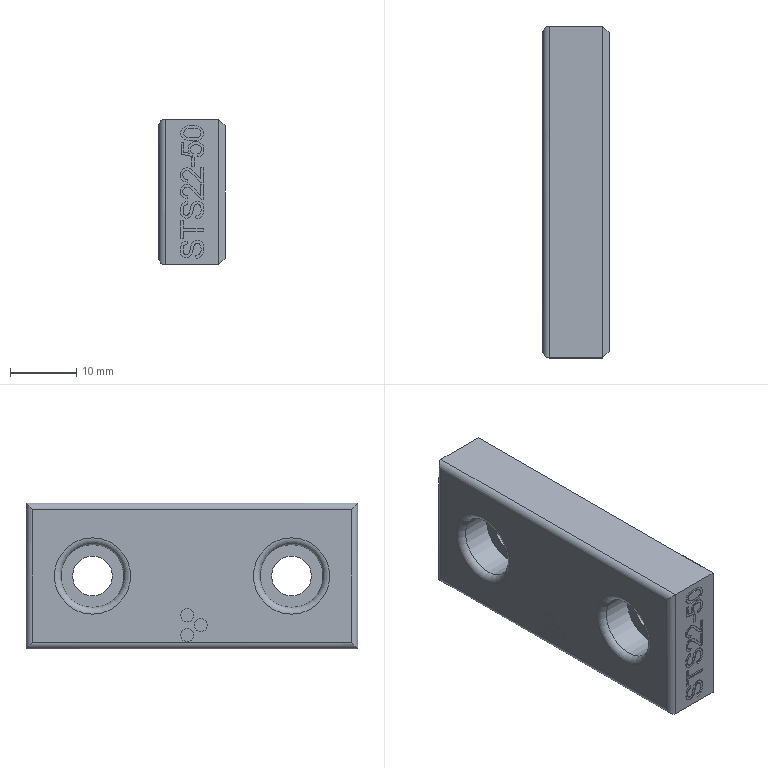Part | STEP file | PN_0064_id202_x_t | 1 solid | 138 faces | box 10.01 x 50 x 22 mm | volume 9849 mm3 | plane 82 | cylinder 54 | torus 2 | commonest cylinder face diameters 2 x7 0.956 x2 0.99 x2 1.313 x2 1.429 x2 1.593 x2